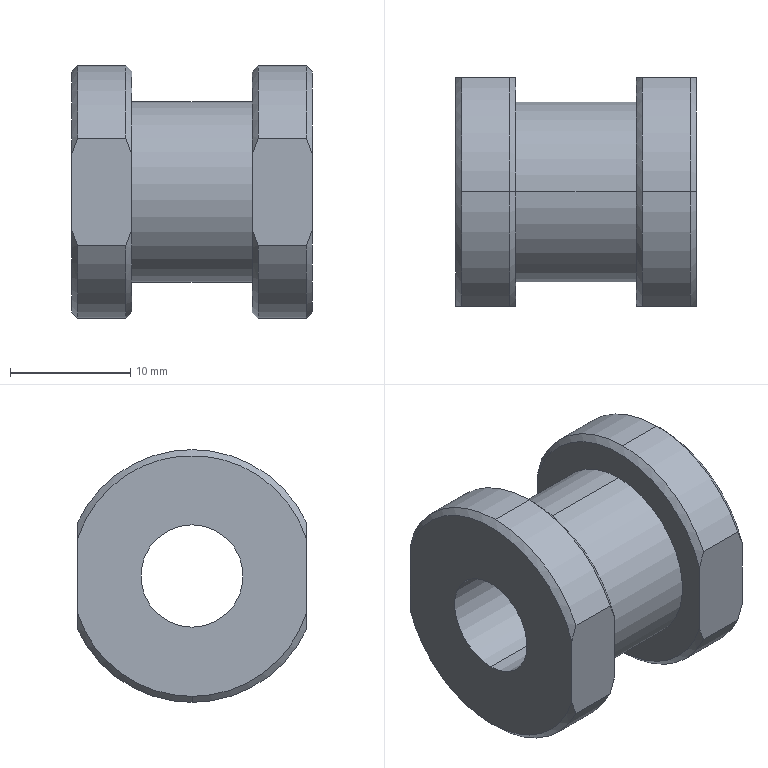Part | STEP file | BPSP-11-12 Pusher Cylinder Connecting Block_Default | 1 solid | 30 faces | box 20 x 19 x 21 mm | volume 3951 mm3 | cone 12 | cylinder 10 | plane 8 | commonest cylinder face diameters 21 x6 8.5 x2 15 x2